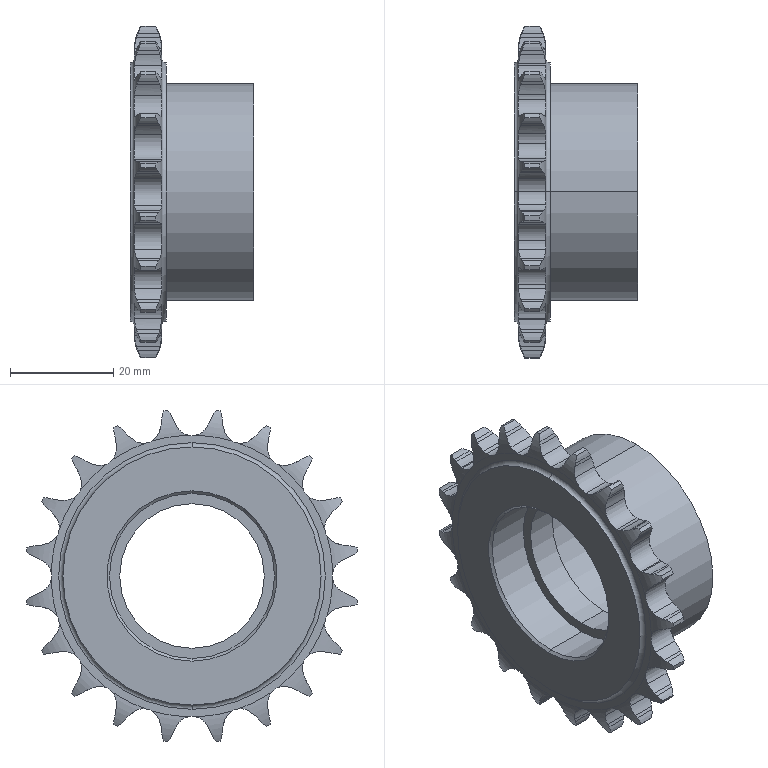Part | STEP file | Driven sprocket_05B | 1 solid | 236 faces | box 24 x 64.324 x 64.324 mm | volume 22666 mm3 | cylinder 141 | plane 47 | torus 44 | cone 4 | commonest cylinder face diameters 9.196 x42 16.642 x42 6.482 x25 65 x20 32 x4 50 x4